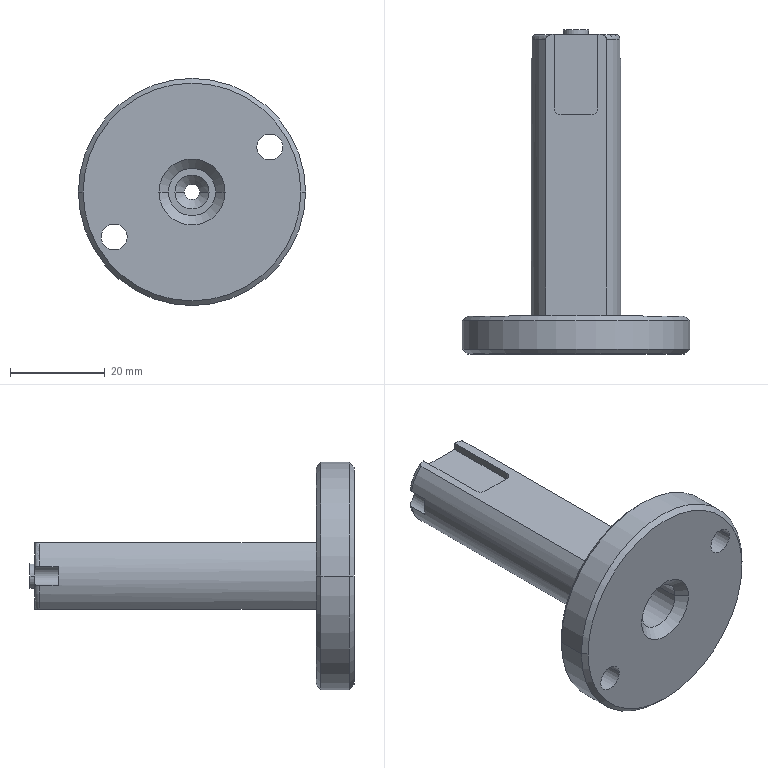Part | STEP file | BU-A06#180 | 1 solid | 54 faces | box 48 x 68.5 x 48 mm | volume 23546 mm3 | cylinder 24 | plane 18 | cone 8 | torus 4 | commonest cylinder face diameters 3 x4 5.5 x4 4 x3 19 x3 3.2 x2 5.3 x2